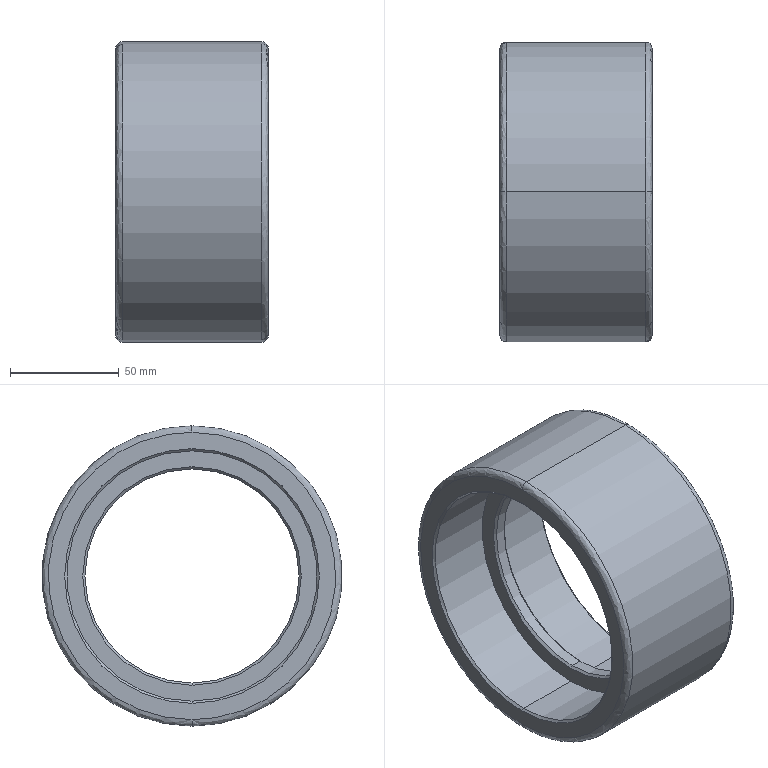Part | SolidWorks | features BaseBody 1 | 1 solid | 24 faces | box 70 x 138 x 138 mm | volume 337126 mm3 | cylinder 8 | cone 8 | spline 4 | plane 4 | commonest cylinder face diameters 115 x4 98.388 x2 138 x2
STEP:
#1=CARTESIAN_POINT('',(15.,-23.981,69.));
#2=VERTEX_POINT('',#1);
#3=CARTESIAN_POINT('',(15.,-23.981,-69.));
#4=VERTEX_POINT('',#3);
#5=CARTESIAN_POINT('',(15.,-23.981,0.));
#6=DIRECTION('',(1.,0.,0.));
#7=DIRECTION('',(0.,0.,-1.));
#8=AXIS2_PLACEMENT_3D('',#5,#6,#7);
#9=CIRCLE('',#8,69.);
#10=EDGE_CURVE('',#2,#4,#9,.T.);
#11=ORIENTED_EDGE('',*,*,#10,.F.);
#12=CARTESIAN_POINT('',(12.,-23.981,66.));
#13=VERTEX_POINT('',#12);
#14=CARTESIAN_POINT('',(15.,-23.981,66.));
#15=DIRECTION('',(0.,-1.,0.));
#16=DIRECTION('',(0.,0.,1.));
#17=AXIS2_PLACEMENT_3D('',#14,#15,#16);
#18=CIRCLE('',#17,3.);
#19=EDGE_CURVE('',#2,#13,#18,.T.);
#20=ORIENTED_EDGE('',*,*,#19,.T.);
#21=CARTESIAN_POINT('',(12.,-23.981,-66.));
#22=VERTEX_POINT('',#21);
#23=CARTESIAN_POINT('',(12.,-23.981,66.));
#24=CARTESIAN_POINT('',(12.,-155.981,66.));
#25=CARTESIAN_POINT('',(12.,-155.981,-66.));
#26=CARTESIAN_POINT('',(12.,-23.981,-66.));
#27=(BOUNDED_CURVE()B_SPLINE_CURVE(3,(#23,#24,#25,#26),.UNSPECIFIED.,.F.,.T.)B_SPLINE_CURVE_WITH_KNOTS((4,4),(0.25,0.75),.UNSPECIFIED.)CURVE()GEOMETRIC_REPRESENTATION_ITEM()RATIONAL_B_SPLINE_CURVE((1.,0.3333,0.3333,1.))REPRESENTATION_ITEM(''));
#28=EDGE_CURVE('',#13,#22,#27,.T.);
#29=ORIENTED_EDGE('',*,*,#28,.T.);
#30=CARTESIAN_POINT('',(15.,-23.981,-66.));
#31=DIRECTION('',(0.,1.,0.));
#32=DIRECTION('',(0.,0.,-1.));
#33=AXIS2_PLACEMENT_3D('',#30,#31,#32);
#34=CIRCLE('',#33,3.);
#35=EDGE_CURVE('',#4,#22,#34,.T.);
#36=ORIENTED_EDGE('',*,*,#35,.F.);
#37=EDGE_LOOP('',(#11,#20,#29,#36));
#38=FACE_OUTER_BOUND('',#37,.T.);
#39=CARTESIAN_POINT('',(15.,-23.981,69.));
#40=CARTESIAN_POINT('',(15.,-161.981,69.));
#41=CARTESIAN_POINT('',(15.,-161.981,-69.));
#42=CARTESIAN_POINT('',(15.,-23.981,-69.));
#43=CARTESIAN_POINT('',(13.243,-23.981,69.));
#44=CARTESIAN_POINT('',(13.243,-161.981,69.));
#45=CARTESIAN_POINT('',(13.243,-161.981,-69.));
#46=CARTESIAN_POINT('',(13.243,-23.981,-69.));
#47=CARTESIAN_POINT('',(12.,-23.981,67.757));
#48=CARTESIAN_POINT('',(12.,-159.495,67.757));
#49=CARTESIAN_POINT('',(12.,-159.495,-67.757));
#50=CARTESIAN_POINT('',(12.,-23.981,-67.757));
#51=CARTESIAN_POINT('',(12.,-23.981,66.));
#52=CARTESIAN_POINT('',(12.,-155.981,66.));
#53=CARTESIAN_POINT('',(12.,-155.981,-66.));
#54=CARTESIAN_POINT('',(12.,-23.981,-66.));
#55=(BOUNDED_SURFACE()B_SPLINE_SURFACE(3,3,((#39,#40,#41,#42),(#43,#44,#45,#46),(#47,#48,#49,#50),(#51,#52,#53,#54)),.UNSPECIFIED.,.F.,.F.,.F.)B_SPLINE_SURFACE_WITH_KNOTS((4,4),(4,4),(0.,1.),(0.,1.),.UNSPECIFIED.)GEOMETRIC_REPRESENTATION_ITEM()RATIONAL_B_SPLINE_SURFACE(((1.,0.3333,0.3333,1.),(0.8047,0.2682,0.2682,0.8047),(0.8047,0.2682,0.2682,0.8047),(1.,0.3333,0.3333,1.)))REPRESENTATION_ITEM('')SURFACE());
#56=ADVANCED_FACE('',(#38),#55,.T.);
#57=CARTESIAN_POINT('',(82.,-23.981,-66.));
#58=VERTEX_POINT('',#57);
#59=CARTESIAN_POINT('',(82.,-23.981,66.));
#60=VERTEX_POINT('',#59);
#61=CARTESIAN_POINT('',(82.,-23.981,-66.));
#62=CARTESIAN_POINT('',(82.,-155.981,-66.));
#63=CARTESIAN_POINT('',(82.,-155.981,66.));
#64=CARTESIAN_POINT('',(82.,-23.981,66.));
#65=(BOUNDED_CURVE()B_SPLINE_CURVE(3,(#61,#62,#63,#64),.UNSPECIFIED.,.F.,.T.)B_SPLINE_CURVE_WITH_KNOTS((4,4),(0.25,0.75),.UNSPECIFIED.)CURVE()GEOMETRIC_REPRESENTATION_ITEM()RATIONAL_B_SPLINE_CURVE((1.,0.3333,0.3333,1.))REPRESENTATION_ITEM(''));
#66=EDGE_CURVE('',#58,#60,#65,.T.);
#67=ORIENTED_EDGE('',*,*,#66,.T.);
#68=CARTESIAN_POINT('',(79.,-23.981,69.));
#69=VERTEX_POINT('',#68);
#70=CARTESIAN_POINT('',(79.,-23.981,66.));
#71=DIRECTION('',(0.,-1.,0.));
#72=DIRECTION('',(0.,0.,1.));
#73=AXIS2_PLACEMENT_3D('',#70,#71,#72);
#74=CIRCLE('',#73,3.);
#75=EDGE_CURVE('',#60,#69,#74,.T.);
#76=ORIENTED_EDGE('',*,*,#75,.T.);
#77=CARTESIAN_POINT('',(79.,-23.981,-69.));
#78=VERTEX_POINT('',#77);
#79=CARTESIAN_POINT('',(79.,-23.981,0.));
#80=DIRECTION('',(-1.,0.,0.));
#81=DIRECTION('',(0.,0.,-1.));
#82=AXIS2_PLACEMENT_3D('',#79,#80,#81);
#83=CIRCLE('',#82,69.);
#84=EDGE_CURVE('',#78,#69,#83,.T.);
#85=ORIENTED_EDGE('',*,*,#84,.F.);
#86=CARTESIAN_POINT('',(79.,-23.981,-66.));
#87=DIRECTION('',(0.,1.,0.));
#88=DIRECTION('',(0.,0.,-1.));
#89=AXIS2_PLACEMENT_3D('',#86,#87,#88);
#90=CIRCLE('',#89,3.);
#91=EDGE_CURVE('',#58,#78,#90,.T.);
#92=ORIENTED_EDGE('',*,*,#91,.F.);
#93=EDGE_LOOP('',(#67,#76,#85,#92));
#94=FACE_OUTER_BOUND('',#93,.T.);
#95=CARTESIAN_POINT('',(82.,-23.981,66.));
#96=CARTESIAN_POINT('',(82.,-155.981,66.));
#97=CARTESIAN_POINT('',(82.,-155.981,-66.));
#98=CARTESIAN_POINT('',(82.,-23.981,-66.));
#99=CARTESIAN_POINT('',(82.,-23.981,67.757));
#100=CARTESIAN_POINT('',(82.,-159.495,67.757));
#101=CARTESIAN_POINT('',(82.,-159.495,-67.757));
#102=CARTESIAN_POINT('',(82.,-23.981,-67.757));
#103=CARTESIAN_POINT('',(80.758,-23.981,69.));
#104=CARTESIAN_POINT('',(80.758,-161.981,69.));
#105=CARTESIAN_POINT('',(80.758,-161.981,-69.));
#106=CARTESIAN_POINT('',(80.758,-23.981,-69.));
#107=CARTESIAN_POINT('',(79.,-23.981,69.));
#108=CARTESIAN_POINT('',(79.,-161.981,69.));
#109=CARTESIAN_POINT('',(79.,-161.981,-69.));
#110=CARTESIAN_POINT('',(79.,-23.981,-69.));
#111=(BOUNDED_SURFACE()B_SPLINE_SURFACE(3,3,((#95,#96,#97,#98),(#99,#100,#101,#102),(#103,#104,#105,#106),(#107,#108,#109,#110)),.UNSPECIFIED.,.F.,.F.,.T.)B_SPLINE_SURFACE_WITH_KNOTS((4,4),(4,4),(0.,1.),(0.,1.),.UNSPECIFIED.)GEOMETRIC_REPRESENTATION_ITEM()RATIONAL_B_SPLINE_SURFACE(((1.,0.3333,0.3333,1.),(0.8047,0.2682,0.2682,0.8047),(0.8047,0.2682,0.2682,0.8047),(1.,0.3333,0.3333,1.)))REPRESENTATION_ITEM('')SURFACE());
#112=ADVANCED_FACE('',(#94),#111,.T.);
#113=CARTESIAN_POINT('',(15.,-23.981,0.));
#114=DIRECTION('',(1.,0.,0.));
#115=DIRECTION('',(0.,0.,-1.));
#116=AXIS2_PLACEMENT_3D('',#113,#114,#115);
#117=CIRCLE('',#116,69.);
#118=EDGE_CURVE('',#4,#2,#117,.T.);
#119=ORIENTED_EDGE('',*,*,#118,.T.);
#120=CARTESIAN_POINT('',(47.,-23.981,69.));
#121=DIRECTION('',(1.,0.,0.));
#122=VECTOR('',#121,1000.);
#123=LINE('',#120,#122);
#124=EDGE_CURVE('',#2,#69,#123,.T.);
#125=ORIENTED_EDGE('',*,*,#124,.T.);
#126=CARTESIAN_POINT('',(79.,-23.981,0.));
#127=DIRECTION('',(-1.,0.,0.));
#128=DIRECTION('',(0.,0.,-1.));
#129=AXIS2_PLACEMENT_3D('',#126,#127,#128);
#130=CIRCLE('',#129,69.);
#131=EDGE_CURVE('',#69,#78,#130,.T.);
#132=ORIENTED_EDGE('',*,*,#131,.T.);
#133=CARTESIAN_POINT('',(47.,-23.981,-69.));
#134=DIRECTION('',(1.,0.,0.));
#135=VECTOR('',#134,1000.);
#136=LINE('',#133,#135);
#137=EDGE_CURVE('',#4,#78,#136,.T.);
#138=ORIENTED_EDGE('',*,*,#137,.F.);
#139=EDGE_LOOP('',(#119,#125,#132,#138));
#140=FACE_OUTER_BOUND('',#139,.T.);
#141=CARTESIAN_POINT('',(47.,-23.981,0.));
#142=DIRECTION('',(1.,0.,0.));
#143=DIRECTION('',(0.,0.,-1.));
#144=AXIS2_PLACEMENT_3D('',#141,#142,#143);
#145=CYLINDRICAL_SURFACE('',#144,69.);
#146=ADVANCED_FACE('',(#140),#145,.T.);
#147=CARTESIAN_POINT('',(13.,-23.981,-57.5));
#148=VERTEX_POINT('',#147);
#149=CARTESIAN_POINT('',(13.,-23.981,57.5));
#150=VERTEX_POINT('',#149);
#151=CARTESIAN_POINT('',(13.,-23.981,0.));
#152=DIRECTION('',(-1.,0.,0.));
#153=DIRECTION('',(0.,-1.,0.));
#154=AXIS2_PLACEMENT_3D('',#151,#152,#153);
#155=CIRCLE('',#154,57.5);
#156=EDGE_CURVE('',#148,#150,#155,.T.);
#157=ORIENTED_EDGE('',*,*,#156,.F.);
#158=CARTESIAN_POINT('',(12.,-23.981,-58.5));
#159=VERTEX_POINT('',#158);
#160=CARTESIAN_POINT('',(12.,-23.981,-58.5));
#161=DIRECTION('',(-0.7071,0.,-0.7071));
#162=VECTOR('',#161,1000.);
#163=LINE('',#160,#162);
#164=EDGE_CURVE('',#148,#159,#163,.T.);
#165=ORIENTED_EDGE('',*,*,#164,.T.);
#166=CARTESIAN_POINT('',(12.,-23.981,58.5));
#167=VERTEX_POINT('',#166);
#168=CARTESIAN_POINT('',(12.,-23.981,0.));
#169=DIRECTION('',(1.,0.,0.));
#170=DIRECTION('',(0.,0.,1.));
#171=AXIS2_PLACEMENT_3D('',#168,#169,#170);
#172=CIRCLE('',#171,58.5);
#173=EDGE_CURVE('',#167,#159,#172,.T.);
#174=ORIENTED_EDGE('',*,*,#173,.F.);
#175=CARTESIAN_POINT('',(12.,-23.981,58.5));
#176=DIRECTION('',(-0.7071,0.,0.7071));
#177=VECTOR('',#176,1000.);
#178=LINE('',#175,#177);
#179=EDGE_CURVE('',#150,#167,#178,.T.);
#180=ORIENTED_EDGE('',*,*,#179,.F.);
#181=EDGE_LOOP('',(#157,#165,#174,#180));
#182=FACE_OUTER_BOUND('',#181,.T.);
#183=CARTESIAN_POINT('',(12.,-23.981,0.));
#184=DIRECTION('',(-1.,0.,0.));
#185=DIRECTION('',(0.,0.,1.));
#186=AXIS2_PLACEMENT_3D('',#183,#184,#185);
#187=CONICAL_SURFACE('',#186,58.5,0.7854);
#188=ADVANCED_FACE('',(#182),#187,.F.);
#189=CARTESIAN_POINT('',(81.,-23.981,57.5));
#190=VERTEX_POINT('',#189);
#191=CARTESIAN_POINT('',(81.,-23.981,-57.5));
#192=VERTEX_POINT('',#191);
#193=CARTESIAN_POINT('',(81.,-23.981,0.));
#194=DIRECTION('',(1.,0.,0.));
#195=DIRECTION('',(0.,-1.,0.));
#196=AXIS2_PLACEMENT_3D('',#193,#194,#195);
#197=CIRCLE('',#196,57.5);
#198=EDGE_CURVE('',#190,#192,#197,.T.);
#199=ORIENTED_EDGE('',*,*,#198,.F.);
#200=CARTESIAN_POINT('',(82.,-23.981,58.5));
#201=VERTEX_POINT('',#200);
#202=CARTESIAN_POINT('',(82.,-23.981,58.5));
#203=DIRECTION('',(0.7071,0.,0.7071));
#204=VECTOR('',#203,1000.);
#205=LINE('',#202,#204);
#206=EDGE_CURVE('',#190,#201,#205,.T.);
#207=ORIENTED_EDGE('',*,*,#206,.T.);
#208=CARTESIAN_POINT('',(82.,-23.981,-58.5));
#209=VERTEX_POINT('',#208);
#210=CARTESIAN_POINT('',(82.,-23.981,0.));
#211=DIRECTION('',(-1.,0.,0.));
#212=DIRECTION('',(0.,0.,-1.));
#213=AXIS2_PLACEMENT_3D('',#210,#211,#212);
#214=CIRCLE('',#213,58.5);
#215=EDGE_CURVE('',#209,#201,#214,.T.);
#216=ORIENTED_EDGE('',*,*,#215,.F.);
#217=CARTESIAN_POINT('',(82.,-23.981,-58.5));
#218=DIRECTION('',(0.7071,0.,-0.7071));
#219=VECTOR('',#218,1000.);
#220=LINE('',#217,#219);
#221=EDGE_CURVE('',#192,#209,#220,.T.);
#222=ORIENTED_EDGE('',*,*,#221,.F.);
#223=EDGE_LOOP('',(#199,#207,#216,#222));
#224=FACE_OUTER_BOUND('',#223,.T.);
#225=CARTESIAN_POINT('',(82.,-23.981,0.));
#226=DIRECTION('',(1.,0.,0.));
#227=DIRECTION('',(0.,0.,-1.));
#228=AXIS2_PLACEMENT_3D('',#225,#226,#227);
#229=CONICAL_SURFACE('',#228,58.5,0.7854);
#230=ADVANCED_FACE('',(#224),#229,.F.);
#231=ORIENTED_EDGE('',*,*,#156,.T.);
#232=CARTESIAN_POINT('',(43.5,-23.981,57.5));
#233=VERTEX_POINT('',#232);
#234=CARTESIAN_POINT('',(27.75,-23.981,57.5));
#235=DIRECTION('',(1.,0.,0.));
#236=VECTOR('',#235,1000.);
#237=LINE('',#234,#236);
#238=EDGE_CURVE('',#150,#233,#237,.T.);
#239=ORIENTED_EDGE('',*,*,#238,.T.);
#240=CARTESIAN_POINT('',(43.5,-23.981,-57.5));
#241=VERTEX_POINT('',#240);
#242=CARTESIAN_POINT('',(43.5,-23.981,0.));
#243=DIRECTION('',(-1.,0.,0.));
#244=DIRECTION('',(0.,0.,-1.));
#245=AXIS2_PLACEMENT_3D('',#242,#243,#244);
#246=CIRCLE('',#245,57.5);
#247=EDGE_CURVE('',#241,#233,#246,.T.);
#248=ORIENTED_EDGE('',*,*,#247,.F.);
#249=CARTESIAN_POINT('',(27.75,-23.981,-57.5));
#250=DIRECTION('',(1.,0.,0.));
#251=VECTOR('',#250,1000.);
#252=LINE('',#249,#251);
#253=EDGE_CURVE('',#148,#241,#252,.T.);
#254=ORIENTED_EDGE('',*,*,#253,.F.);
#255=EDGE_LOOP('',(#231,#239,#248,#254));
#256=FACE_OUTER_BOUND('',#255,.T.);
#257=CARTESIAN_POINT('',(27.75,-23.981,0.));
#258=DIRECTION('',(1.,0.,0.));
#259=DIRECTION('',(0.,0.,-1.));
#260=AXIS2_PLACEMENT_3D('',#257,#258,#259);
#261=CYLINDRICAL_SURFACE('',#260,57.5);
#262=ADVANCED_FACE('',(#256),#261,.F.);
#263=CARTESIAN_POINT('',(50.5,-23.981,57.5));
#264=VERTEX_POINT('',#263);
#265=CARTESIAN_POINT('',(50.5,-23.981,-57.5));
#266=VERTEX_POINT('',#265);
#267=CARTESIAN_POINT('',(50.5,-23.981,0.));
#268=DIRECTION('',(1.,0.,0.));
#269=DIRECTION('',(0.,0.,-1.));
#270=AXIS2_PLACEMENT_3D('',#267,#268,#269);
#271=CIRCLE('',#270,57.5);
#272=EDGE_CURVE('',#264,#266,#271,.T.);
#273=ORIENTED_EDGE('',*,*,#272,.F.);
#274=CARTESIAN_POINT('',(51.25,-23.981,57.5));
#275=DIRECTION('',(1.,0.,0.));
#276=VECTOR('',#275,1000.);
#277=LINE('',#274,#276);
#278=EDGE_CURVE('',#264,#190,#277,.T.);
#279=ORIENTED_EDGE('',*,*,#278,.T.);
#280=ORIENTED_EDGE('',*,*,#198,.T.);
#281=CARTESIAN_POINT('',(51.25,-23.981,-57.5));
#282=DIRECTION('',(1.,0.,0.));
#283=VECTOR('',#282,1000.);
#284=LINE('',#281,#283);
#285=EDGE_CURVE('',#266,#192,#284,.T.);
#286=ORIENTED_EDGE('',*,*,#285,.F.);
#287=EDGE_LOOP('',(#273,#279,#280,#286));
#288=FACE_OUTER_BOUND('',#287,.T.);
#289=CARTESIAN_POINT('',(51.25,-23.981,0.));
#290=DIRECTION('',(1.,0.,0.));
#291=DIRECTION('',(0.,0.,-1.));
#292=AXIS2_PLACEMENT_3D('',#289,#290,#291);
#293=CYLINDRICAL_SURFACE('',#292,57.5);
#294=ADVANCED_FACE('',(#288),#293,.F.);
#295=CARTESIAN_POINT('',(44.5,-23.981,-49.194));
#296=VERTEX_POINT('',#295);
#297=CARTESIAN_POINT('',(44.5,-23.981,49.194));
#298=VERTEX_POINT('',#297);
#299=CARTESIAN_POINT('',(44.5,-23.981,0.));
#300=DIRECTION('',(-1.,0.,0.));
#301=DIRECTION('',(0.,-1.,0.));
#302=AXIS2_PLACEMENT_3D('',#299,#300,#301);
#303=CIRCLE('',#302,49.194);
#304=EDGE_CURVE('',#296,#298,#303,.T.);
#305=ORIENTED_EDGE('',*,*,#304,.F.);
#306=CARTESIAN_POINT('',(43.5,-23.981,-50.194));
#307=VERTEX_POINT('',#306);
#308=CARTESIAN_POINT('',(43.5,-23.981,-50.194));
#309=DIRECTION('',(-0.7071,0.,-0.7071));
#310=VECTOR('',#309,1000.);
#311=LINE('',#308,#310);
#312=EDGE_CURVE('',#296,#307,#311,.T.);
#313=ORIENTED_EDGE('',*,*,#312,.T.);
#314=CARTESIAN_POINT('',(43.5,-23.981,50.194));
#315=VERTEX_POINT('',#314);
#316=CARTESIAN_POINT('',(43.5,-23.981,0.));
#317=DIRECTION('',(1.,0.,0.));
#318=DIRECTION('',(0.,0.,1.));
#319=AXIS2_PLACEMENT_3D('',#316,#317,#318);
#320=CIRCLE('',#319,50.194);
#321=EDGE_CURVE('',#315,#307,#320,.T.);
#322=ORIENTED_EDGE('',*,*,#321,.F.);
#323=CARTESIAN_POINT('',(43.5,-23.981,50.194));
#324=DIRECTION('',(-0.7071,0.,0.7071));
#325=VECTOR('',#324,1000.);
#326=LINE('',#323,#325);
#327=EDGE_CURVE('',#298,#315,#326,.T.);
#328=ORIENTED_EDGE('',*,*,#327,.F.);
#329=EDGE_LOOP('',(#305,#313,#322,#328));
#330=FACE_OUTER_BOUND('',#329,.T.);
#331=CARTESIAN_POINT('',(43.5,-23.981,0.));
#332=DIRECTION('',(-1.,0.,0.));
#333=DIRECTION('',(0.,0.,1.));
#334=AXIS2_PLACEMENT_3D('',#331,#332,#333);
#335=CONICAL_SURFACE('',#334,50.194,0.7854);
#336=ADVANCED_FACE('',(#330),#335,.F.);
#337=CARTESIAN_POINT('',(49.5,-23.981,49.194));
#338=VERTEX_POINT('',#337);
#339=CARTESIAN_POINT('',(49.5,-23.981,-49.194));
#340=VERTEX_POINT('',#339);
#341=CARTESIAN_POINT('',(49.5,-23.981,0.));
#342=DIRECTION('',(1.,0.,0.));
#343=DIRECTION('',(0.,-1.,0.));
#344=AXIS2_PLACEMENT_3D('',#341,#342,#343);
#345=CIRCLE('',#344,49.194);
#346=EDGE_CURVE('',#338,#340,#345,.T.);
#347=ORIENTED_EDGE('',*,*,#346,.F.);
#348=CARTESIAN_POINT('',(50.5,-23.981,50.194));
#349=VERTEX_POINT('',#348);
#350=CARTESIAN_POINT('',(50.5,-23.981,50.194));
#351=DIRECTION('',(0.7071,0.,0.7071));
#352=VECTOR('',#351,1000.);
#353=LINE('',#350,#352);
#354=EDGE_CURVE('',#338,#349,#353,.T.);
#355=ORIENTED_EDGE('',*,*,#354,.T.);
#356=CARTESIAN_POINT('',(50.5,-23.981,-50.194));
#357=VERTEX_POINT('',#356);
#358=CARTESIAN_POINT('',(50.5,-23.981,0.));
#359=DIRECTION('',(-1.,0.,0.));
#360=DIRECTION('',(0.,0.,-1.));
#361=AXIS2_PLACEMENT_3D('',#358,#359,#360);
#362=CIRCLE('',#361,50.194);
#363=EDGE_CURVE('',#357,#349,#362,.T.);
#364=ORIENTED_EDGE('',*,*,#363,.F.);
#365=CARTESIAN_POINT('',(50.5,-23.981,-50.194));
#366=DIRECTION('',(0.7071,0.,-0.7071));
#367=VECTOR('',#366,1000.);
#368=LINE('',#365,#367);
#369=EDGE_CURVE('',#340,#357,#368,.T.);
#370=ORIENTED_EDGE('',*,*,#369,.F.);
#371=EDGE_LOOP('',(#347,#355,#364,#370));
#372=FACE_OUTER_BOUND('',#371,.T.);
#373=CARTESIAN_POINT('',(50.5,-23.981,0.));
#374=DIRECTION('',(1.,0.,0.));
#375=DIRECTION('',(0.,0.,-1.));
#376=AXIS2_PLACEMENT_3D('',#373,#374,#375);
#377=CONICAL_SURFACE('',#376,50.194,0.7854);
#378=ADVANCED_FACE('',(#372),#377,.F.);
#379=ORIENTED_EDGE('',*,*,#304,.T.);
#380=CARTESIAN_POINT('',(47.,-23.981,49.194));
#381=DIRECTION('',(1.,0.,0.));
#382=VECTOR('',#381,1000.);
#383=LINE('',#380,#382);
#384=EDGE_CURVE('',#298,#338,#383,.T.);
#385=ORIENTED_EDGE('',*,*,#384,.T.);
#386=ORIENTED_EDGE('',*,*,#346,.T.);
#387=CARTESIAN_POINT('',(47.,-23.981,-49.194));
#388=DIRECTION('',(1.,0.,0.));
#389=VECTOR('',#388,1000.);
#390=LINE('',#387,#389);
#391=EDGE_CURVE('',#296,#340,#390,.T.);
#392=ORIENTED_EDGE('',*,*,#391,.F.);
#393=EDGE_LOOP('',(#379,#385,#386,#392));
#394=FACE_OUTER_BOUND('',#393,.T.);
#395=CARTESIAN_POINT('',(47.,-23.981,0.));
#396=DIRECTION('',(1.,0.,0.));
#397=DIRECTION('',(0.,0.,-1.));
#398=AXIS2_PLACEMENT_3D('',#395,#396,#397);
#399=CYLINDRICAL_SURFACE('',#398,49.194);
#400=ADVANCED_FACE('',(#394),#399,.F.);
#401=ORIENTED_EDGE('',*,*,#124,.F.);
#402=ORIENTED_EDGE('',*,*,#10,.T.);
#403=ORIENTED_EDGE('',*,*,#137,.T.);
#404=ORIENTED_EDGE('',*,*,#84,.T.);
#405=EDGE_LOOP('',(#401,#402,#403,#404));
#406=FACE_OUTER_BOUND('',#405,.T.);
#407=CARTESIAN_POINT('',(47.,-23.981,0.));
#408=DIRECTION('',(1.,0.,0.));
#409=DIRECTION('',(0.,0.,-1.));
#410=AXIS2_PLACEMENT_3D('',#407,#408,#409);
#411=CYLINDRICAL_SURFACE('',#410,69.);
#412=ADVANCED_FACE('',(#406),#411,.T.);
#413=ORIENTED_EDGE('',*,*,#19,.F.);
#414=ORIENTED_EDGE('',*,*,#118,.F.);
#415=ORIENTED_EDGE('',*,*,#35,.T.);
#416=CARTESIAN_POINT('',(12.,-23.981,-66.));
#417=CARTESIAN_POINT('',(12.,108.019,-66.));
#418=CARTESIAN_POINT('',(12.,108.019,66.));
#419=CARTESIAN_POINT('',(12.,-23.981,66.));
#420=(BOUNDED_CURVE()B_SPLINE_CURVE(3,(#416,#417,#418,#419),.UNSPECIFIED.,.F.,.T.)B_SPLINE_CURVE_WITH_KNOTS((4,4),(0.75,1.25),.UNSPECIFIED.)CURVE()GEOMETRIC_REPRESENTATION_ITEM()RATIONAL_B_SPLINE_CURVE((1.,0.3333,0.3333,1.))REPRESENTATION_ITEM(''));
#421=EDGE_CURVE('',#22,#13,#420,.T.);
#422=ORIENTED_EDGE('',*,*,#421,.T.);
#423=EDGE_LOOP('',(#413,#414,#415,#422));
#424=FACE_OUTER_BOUND('',#423,.T.);
#425=CARTESIAN_POINT('',(15.,-23.981,-69.));
#426=CARTESIAN_POINT('',(15.,114.019,-69.));
#427=CARTESIAN_POINT('',(15.,114.019,69.));
#428=CARTESIAN_POINT('',(15.,-23.981,69.));
#429=CARTESIAN_POINT('',(13.243,-23.981,-69.));
#430=CARTESIAN_POINT('',(13.243,114.019,-69.));
#431=CARTESIAN_POINT('',(13.243,114.019,69.));
#432=CARTESIAN_POINT('',(13.243,-23.981,69.));
#433=CARTESIAN_POINT('',(12.,-23.981,-67.757));
#434=CARTESIAN_POINT('',(12.,111.534,-67.757));
#435=CARTESIAN_POINT('',(12.,111.534,67.757));
#436=CARTESIAN_POINT('',(12.,-23.981,67.757));
#437=CARTESIAN_POINT('',(12.,-23.981,-66.));
#438=CARTESIAN_POINT('',(12.,108.019,-66.));
#439=CARTESIAN_POINT('',(12.,108.019,66.));
#440=CARTESIAN_POINT('',(12.,-23.981,66.));
#441=(BOUNDED_SURFACE()B_SPLINE_SURFACE(3,3,((#425,#426,#427,#428),(#429,#430,#431,#432),(#433,#434,#435,#436),(#437,#438,#439,#440)),.UNSPECIFIED.,.F.,.F.,.F.)B_SPLINE_SURFACE_WITH_KNOTS((4,4),(4,4),(0.,1.),(0.,1.),.UNSPECIFIED.)GEOMETRIC_REPRESENTATION_ITEM()RATIONAL_B_SPLINE_SURFACE(((1.,0.3333,0.3333,1.),(0.8047,0.2682,0.2682,0.8047),(0.8047,0.2682,0.2682,0.8047),(1.,0.3333,0.3333,1.)))REPRESENTATION_ITEM('')SURFACE());
#442=ADVANCED_FACE('',(#424),#441,.T.);
#443=ORIENTED_EDGE('',*,*,#75,.F.);
#444=CARTESIAN_POINT('',(82.,-23.981,66.));
#445=CARTESIAN_POINT('',(82.,108.019,66.));
#446=CARTESIAN_POINT('',(82.,108.019,-66.));
#447=CARTESIAN_POINT('',(82.,-23.981,-66.));
#448=(BOUNDED_CURVE()B_SPLINE_CURVE(3,(#444,#445,#446,#447),.UNSPECIFIED.,.F.,.T.)B_SPLINE_CURVE_WITH_KNOTS((4,4),(0.75,1.25),.UNSPECIFIED.)CURVE()GEOMETRIC_REPRESENTATION_ITEM()RATIONAL_B_SPLINE_CURVE((1.,0.3333,0.3333,1.))REPRESENTATION_ITEM(''));
#449=EDGE_CURVE('',#60,#58,#448,.T.);
#450=ORIENTED_EDGE('',*,*,#449,.T.);
#451=ORIENTED_EDGE('',*,*,#91,.T.);
#452=ORIENTED_EDGE('',*,*,#131,.F.);
#453=EDGE_LOOP('',(#443,#450,#451,#452));
#454=FACE_OUTER_BOUND('',#453,.T.);
#455=CARTESIAN_POINT('',(82.,-23.981,-66.));
#456=CARTESIAN_POINT('',(82.,108.019,-66.));
#457=CARTESIAN_POINT('',(82.,108.019,66.));
#458=CARTESIAN_POINT('',(82.,-23.981,66.));
#459=CARTESIAN_POINT('',(82.,-23.981,-67.757));
#460=CARTESIAN_POINT('',(82.,111.534,-67.757));
#461=CARTESIAN_POINT('',(82.,111.534,67.757));
#462=CARTESIAN_POINT('',(82.,-23.981,67.757));
#463=CARTESIAN_POINT('',(80.758,-23.981,-69.));
#464=CARTESIAN_POINT('',(80.758,114.019,-69.));
#465=CARTESIAN_POINT('',(80.758,114.019,69.));
#466=CARTESIAN_POINT('',(80.758,-23.981,69.));
#467=CARTESIAN_POINT('',(79.,-23.981,-69.));
#468=CARTESIAN_POINT('',(79.,114.019,-69.));
#469=CARTESIAN_POINT('',(79.,114.019,69.));
#470=CARTESIAN_POINT('',(79.,-23.981,69.));
#471=(BOUNDED_SURFACE()B_SPLINE_SURFACE(3,3,((#455,#456,#457,#458),(#459,#460,#461,#462),(#463,#464,#465,#466),(#467,#468,#469,#470)),.UNSPECIFIED.,.F.,.F.,.F.)B_SPLINE_SURFACE_WITH_KNOTS((4,4),(4,4),(0.,1.),(0.,1.),.UNSPECIFIED.)GEOMETRIC_REPRESENTATION_ITEM()RATIONAL_B_SPLINE_SURFACE(((1.,0.3333,0.3333,1.),(0.8047,0.2682,0.2682,0.8047),(0.8047,0.2682,0.2682,0.8047),(1.,0.3333,0.3333,1.)))REPRESENTATION_ITEM('')SURFACE());
#472=ADVANCED_FACE('',(#454),#471,.T.);
#473=ORIENTED_EDGE('',*,*,#173,.T.);
#474=CARTESIAN_POINT('',(12.,-23.981,0.));
#475=DIRECTION('',(1.,0.,0.));
#476=DIRECTION('',(0.,0.,1.));
#477=AXIS2_PLACEMENT_3D('',#474,#475,#476);
#478=CIRCLE('',#477,58.5);
#479=EDGE_CURVE('',#159,#167,#478,.T.);
#480=ORIENTED_EDGE('',*,*,#479,.T.);
#481=EDGE_LOOP('',(#473,#480));
#482=FACE_BOUND('',#481,.T.);
#483=ORIENTED_EDGE('',*,*,#421,.F.);
#484=ORIENTED_EDGE('',*,*,#28,.F.);
#485=EDGE_LOOP('',(#483,#484));
#486=FACE_OUTER_BOUND('',#485,.T.);
#487=CARTESIAN_POINT('',(12.,39.269,0.));
#488=DIRECTION('',(-1.,0.,0.));
#489=DIRECTION('',(0.,0.,1.));
#490=AXIS2_PLACEMENT_3D('',#487,#488,#489);
#491=PLANE('',#490);
#492=ADVANCED_FACE('',(#482,#486),#491,.T.);
#493=ORIENTED_EDGE('',*,*,#215,.T.);
#494=CARTESIAN_POINT('',(82.,-23.981,0.));
#495=DIRECTION('',(-1.,0.,0.));
#496=DIRECTION('',(0.,0.,-1.));
#497=AXIS2_PLACEMENT_3D('',#494,#495,#496);
#498=CIRCLE('',#497,58.5);
#499=EDGE_CURVE('',#201,#209,#498,.T.);
#500=ORIENTED_EDGE('',*,*,#499,.T.);
#501=EDGE_LOOP('',(#493,#500));
#502=FACE_BOUND('',#501,.T.);
#503=ORIENTED_EDGE('',*,*,#66,.F.);
#504=ORIENTED_EDGE('',*,*,#449,.F.);
#505=EDGE_LOOP('',(#503,#504));
#506=FACE_OUTER_BOUND('',#505,.T.);
#507=CARTESIAN_POINT('',(82.,39.269,0.));
#508=DIRECTION('',(1.,0.,0.));
#509=DIRECTION('',(0.,0.,-1.));
#510=AXIS2_PLACEMENT_3D('',#507,#508,#509);
#511=PLANE('',#510);
#512=ADVANCED_FACE('',(#502,#506),#511,.T.);
#513=ORIENTED_EDGE('',*,*,#164,.F.);
#514=CARTESIAN_POINT('',(13.,-23.981,0.));
#515=DIRECTION('',(-1.,0.,0.));
#516=DIRECTION('',(0.,-1.,0.));
#517=AXIS2_PLACEMENT_3D('',#514,#515,#516);
#518=CIRCLE('',#517,57.5);
#519=EDGE_CURVE('',#150,#148,#518,.T.);
#520=ORIENTED_EDGE('',*,*,#519,.F.);
#521=ORIENTED_EDGE('',*,*,#179,.T.);
#522=ORIENTED_EDGE('',*,*,#479,.F.);
#523=EDGE_LOOP('',(#513,#520,#521,#522));
#524=FACE_OUTER_BOUND('',#523,.T.);
#525=CARTESIAN_POINT('',(12.,-23.981,0.));
#526=DIRECTION('',(-1.,0.,0.));
#527=DIRECTION('',(0.,0.,1.));
#528=AXIS2_PLACEMENT_3D('',#525,#526,#527);
#529=CONICAL_SURFACE('',#528,58.5,0.7854);
#530=ADVANCED_FACE('',(#524),#529,.F.);
#531=ORIENTED_EDGE('',*,*,#206,.F.);
#532=CARTESIAN_POINT('',(81.,-23.981,0.));
#533=DIRECTION('',(1.,0.,0.));
#534=DIRECTION('',(0.,-1.,0.));
#535=AXIS2_PLACEMENT_3D('',#532,#533,#534);
#536=CIRCLE('',#535,57.5);
#537=EDGE_CURVE('',#192,#190,#536,.T.);
#538=ORIENTED_EDGE('',*,*,#537,.F.);
#539=ORIENTED_EDGE('',*,*,#221,.T.);
#540=ORIENTED_EDGE('',*,*,#499,.F.);
#541=EDGE_LOOP('',(#531,#538,#539,#540));
#542=FACE_OUTER_BOUND('',#541,.T.);
#543=CARTESIAN_POINT('',(82.,-23.981,0.));
#544=DIRECTION('',(1.,0.,0.));
#545=DIRECTION('',(0.,0.,-1.));
#546=AXIS2_PLACEMENT_3D('',#543,#544,#545);
#547=CONICAL_SURFACE('',#546,58.5,0.7854);
#548=ADVANCED_FACE('',(#542),#547,.F.);
#549=ORIENTED_EDGE('',*,*,#238,.F.);
#550=ORIENTED_EDGE('',*,*,#519,.T.);
#551=ORIENTED_EDGE('',*,*,#253,.T.);
#552=CARTESIAN_POINT('',(43.5,-23.981,0.));
#553=DIRECTION('',(-1.,0.,0.));
#554=DIRECTION('',(0.,0.,-1.));
#555=AXIS2_PLACEMENT_3D('',#552,#553,#554);
#556=CIRCLE('',#555,57.5);
#557=EDGE_CURVE('',#233,#241,#556,.T.);
#558=ORIENTED_EDGE('',*,*,#557,.F.);
#559=EDGE_LOOP('',(#549,#550,#551,#558));
#560=FACE_OUTER_BOUND('',#559,.T.);
#561=CARTESIAN_POINT('',(27.75,-23.981,0.));
#562=DIRECTION('',(1.,0.,0.));
#563=DIRECTION('',(0.,0.,-1.));
#564=AXIS2_PLACEMENT_3D('',#561,#562,#563);
#565=CYLINDRICAL_SURFACE('',#564,57.5);
#566=ADVANCED_FACE('',(#560),#565,.F.);
#567=ORIENTED_EDGE('',*,*,#278,.F.);
#568=CARTESIAN_POINT('',(50.5,-23.981,0.));
#569=DIRECTION('',(1.,0.,0.));
#570=DIRECTION('',(0.,0.,-1.));
#571=AXIS2_PLACEMENT_3D('',#568,#569,#570);
#572=CIRCLE('',#571,57.5);
#573=EDGE_CURVE('',#266,#264,#572,.T.);
#574=ORIENTED_EDGE('',*,*,#573,.F.);
#575=ORIENTED_EDGE('',*,*,#285,.T.);
#576=ORIENTED_EDGE('',*,*,#537,.T.);
#577=EDGE_LOOP('',(#567,#574,#575,#576));
#578=FACE_OUTER_BOUND('',#577,.T.);
#579=CARTESIAN_POINT('',(51.25,-23.981,0.));
#580=DIRECTION('',(1.,0.,0.));
#581=DIRECTION('',(0.,0.,-1.));
#582=AXIS2_PLACEMENT_3D('',#579,#580,#581);
#583=CYLINDRICAL_SURFACE('',#582,57.5);
#584=ADVANCED_FACE('',(#578),#583,.F.);
#585=ORIENTED_EDGE('',*,*,#321,.T.);
#586=CARTESIAN_POINT('',(43.5,-23.981,0.));
#587=DIRECTION('',(1.,0.,0.));
#588=DIRECTION('',(0.,0.,1.));
#589=AXIS2_PLACEMENT_3D('',#586,#587,#588);
#590=CIRCLE('',#589,50.194);
#591=EDGE_CURVE('',#307,#315,#590,.T.);
#592=ORIENTED_EDGE('',*,*,#591,.T.);
#593=EDGE_LOOP('',(#585,#592));
#594=FACE_BOUND('',#593,.T.);
#595=ORIENTED_EDGE('',*,*,#247,.T.);
#596=ORIENTED_EDGE('',*,*,#557,.T.);
#597=EDGE_LOOP('',(#595,#596));
#598=FACE_OUTER_BOUND('',#597,.T.);
#599=CARTESIAN_POINT('',(43.5,29.366,0.));
#600=DIRECTION('',(-1.,0.,0.));
#601=DIRECTION('',(0.,0.,1.));
#602=AXIS2_PLACEMENT_3D('',#599,#600,#601);
#603=PLANE('',#602);
#604=ADVANCED_FACE('',(#594,#598),#603,.T.);
#605=ORIENTED_EDGE('',*,*,#363,.T.);
#606=CARTESIAN_POINT('',(50.5,-23.981,0.));
#607=DIRECTION('',(-1.,0.,0.));
#608=DIRECTION('',(0.,0.,-1.));
#609=AXIS2_PLACEMENT_3D('',#606,#607,#608);
#610=CIRCLE('',#609,50.194);
#611=EDGE_CURVE('',#349,#357,#610,.T.);
#612=ORIENTED_EDGE('',*,*,#611,.T.);
#613=EDGE_LOOP('',(#605,#612));
#614=FACE_BOUND('',#613,.T.);
#615=ORIENTED_EDGE('',*,*,#573,.T.);
#616=ORIENTED_EDGE('',*,*,#272,.T.);
#617=EDGE_LOOP('',(#615,#616));
#618=FACE_OUTER_BOUND('',#617,.T.);
#619=CARTESIAN_POINT('',(50.5,29.366,0.));
#620=DIRECTION('',(1.,0.,0.));
#621=DIRECTION('',(0.,0.,-1.));
#622=AXIS2_PLACEMENT_3D('',#619,#620,#621);
#623=PLANE('',#622);
#624=ADVANCED_FACE('',(#614,#618),#623,.T.);
#625=ORIENTED_EDGE('',*,*,#312,.F.);
#626=CARTESIAN_POINT('',(44.5,-23.981,0.));
#627=DIRECTION('',(-1.,0.,0.));
#628=DIRECTION('',(0.,-1.,0.));
#629=AXIS2_PLACEMENT_3D('',#626,#627,#628);
#630=CIRCLE('',#629,49.194);
#631=EDGE_CURVE('',#298,#296,#630,.T.);
#632=ORIENTED_EDGE('',*,*,#631,.F.);
#633=ORIENTED_EDGE('',*,*,#327,.T.);
#634=ORIENTED_EDGE('',*,*,#591,.F.);
#635=EDGE_LOOP('',(#625,#632,#633,#634));
#636=FACE_OUTER_BOUND('',#635,.T.);
#637=CARTESIAN_POINT('',(43.5,-23.981,0.));
#638=DIRECTION('',(-1.,0.,0.));
#639=DIRECTION('',(0.,0.,1.));
#640=AXIS2_PLACEMENT_3D('',#637,#638,#639);
#641=CONICAL_SURFACE('',#640,50.194,0.7854);
#642=ADVANCED_FACE('',(#636),#641,.F.);
#643=ORIENTED_EDGE('',*,*,#354,.F.);
#644=CARTESIAN_POINT('',(49.5,-23.981,0.));
#645=DIRECTION('',(1.,0.,0.));
#646=DIRECTION('',(0.,-1.,0.));
#647=AXIS2_PLACEMENT_3D('',#644,#645,#646);
#648=CIRCLE('',#647,49.194);
#649=EDGE_CURVE('',#340,#338,#648,.T.);
#650=ORIENTED_EDGE('',*,*,#649,.F.);
#651=ORIENTED_EDGE('',*,*,#369,.T.);
#652=ORIENTED_EDGE('',*,*,#611,.F.);
#653=EDGE_LOOP('',(#643,#650,#651,#652));
#654=FACE_OUTER_BOUND('',#653,.T.);
#655=CARTESIAN_POINT('',(50.5,-23.981,0.));
#656=DIRECTION('',(1.,0.,0.));
#657=DIRECTION('',(0.,0.,-1.));
#658=AXIS2_PLACEMENT_3D('',#655,#656,#657);
#659=CONICAL_SURFACE('',#658,50.194,0.7854);
#660=ADVANCED_FACE('',(#654),#659,.F.);
#661=ORIENTED_EDGE('',*,*,#384,.F.);
#662=ORIENTED_EDGE('',*,*,#631,.T.);
#663=ORIENTED_EDGE('',*,*,#391,.T.);
#664=ORIENTED_EDGE('',*,*,#649,.T.);
#665=EDGE_LOOP('',(#661,#662,#663,#664));
#666=FACE_OUTER_BOUND('',#665,.T.);
#667=CARTESIAN_POINT('',(47.,-23.981,0.));
#668=DIRECTION('',(1.,0.,0.));
#669=DIRECTION('',(0.,0.,-1.));
#670=AXIS2_PLACEMENT_3D('',#667,#668,#669);
#671=CYLINDRICAL_SURFACE('',#670,49.194);
#672=ADVANCED_FACE('',(#666),#671,.F.);
#673=CLOSED_SHELL('',(#56,#112,#146,#188,#230,#262,#294,#336,#378,#400,#412,#442,#472,#492,#512,#530,#548,#566,#584,#604,#624,#642,#660,#672));
#674=MANIFOLD_SOLID_BREP('',#673);
#675=CARTESIAN_POINT('',(0.,0.,0.));
#676=DIRECTION('',(0.,0.,1.));
#677=DIRECTION('',(1.,0.,0.));
#678=AXIS2_PLACEMENT_3D('',#675,#676,#677);
#679=(LENGTH_UNIT()NAMED_UNIT(*)SI_UNIT(.MILLI.,.METRE.));
#680=UNCERTAINTY_MEASURE_WITH_UNIT(LENGTH_MEASURE(0.00001),#679,'','');
#681=(NAMED_UNIT(*)PLANE_ANGLE_UNIT()SI_UNIT($,.RADIAN.));
#682=(NAMED_UNIT(*)SI_UNIT($,.STERADIAN.)SOLID_ANGLE_UNIT());
#683=(GEOMETRIC_REPRESENTATION_CONTEXT(3)GLOBAL_UNCERTAINTY_ASSIGNED_CONTEXT((#680))GLOBAL_UNIT_ASSIGNED_CONTEXT((#679,#681,#682))REPRESENTATION_CONTEXT('',''));
#684=ADVANCED_BREP_SHAPE_REPRESENTATION('',(#674,#678),#683);